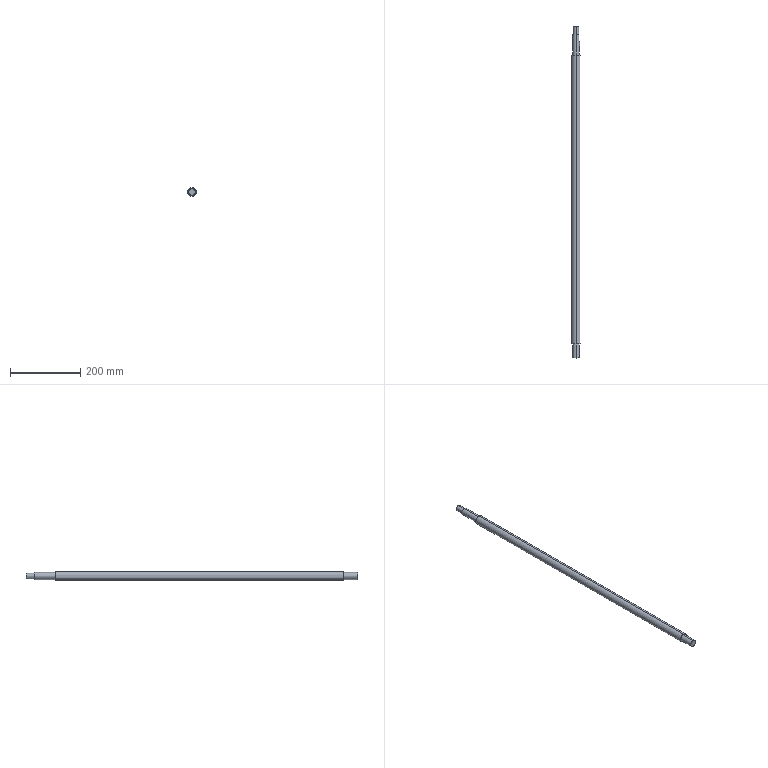Part | STEP file | OT2025004-02-10 Shaft 2 | 1 solid | 28 faces | box 25 x 946 x 25 mm | volume 439586 mm3 | cylinder 12 | cone 9 | plane 7 | commonest cylinder face diameters 2.5 x4 20 x4 16 x2 25 x2
STEP:
#1=CARTESIAN_POINT('',(-0.5,878.75,1.25));
#2=VERTEX_POINT('',#1);
#3=CARTESIAN_POINT('',(-0.5,878.75,-1.25));
#4=VERTEX_POINT('',#3);
#5=CARTESIAN_POINT('',(-0.5,878.75,0.));
#6=DIRECTION('',(1.,0.,0.));
#7=DIRECTION('',(0.,0.,-1.));
#8=AXIS2_PLACEMENT_3D('',#5,#6,#7);
#9=CIRCLE('',#8,1.25);
#10=EDGE_CURVE('',#2,#4,#9,.T.);
#11=ORIENTED_EDGE('',*,*,#10,.F.);
#12=CARTESIAN_POINT('',(8.,878.75,1.25));
#13=VERTEX_POINT('',#12);
#14=CARTESIAN_POINT('',(8.,878.75,1.25));
#15=DIRECTION('',(1.,0.,0.));
#16=VECTOR('',#15,1000.);
#17=LINE('',#14,#16);
#18=EDGE_CURVE('',#2,#13,#17,.T.);
#19=ORIENTED_EDGE('',*,*,#18,.T.);
#20=CARTESIAN_POINT('',(8.,878.75,-1.25));
#21=VERTEX_POINT('',#20);
#22=CARTESIAN_POINT('',(8.,878.75,0.));
#23=DIRECTION('',(1.,0.,0.));
#24=DIRECTION('',(0.,0.,-1.));
#25=AXIS2_PLACEMENT_3D('',#22,#23,#24);
#26=CIRCLE('',#25,1.25);
#27=EDGE_CURVE('',#13,#21,#26,.T.);
#28=ORIENTED_EDGE('',*,*,#27,.T.);
#29=CARTESIAN_POINT('',(8.,878.75,-1.25));
#30=DIRECTION('',(1.,0.,0.));
#31=VECTOR('',#30,1000.);
#32=LINE('',#29,#31);
#33=EDGE_CURVE('',#4,#21,#32,.T.);
#34=ORIENTED_EDGE('',*,*,#33,.F.);
#35=EDGE_LOOP('',(#11,#19,#28,#34));
#36=FACE_OUTER_BOUND('',#35,.T.);
#37=CARTESIAN_POINT('',(8.,878.75,0.));
#38=DIRECTION('',(1.,0.,0.));
#39=DIRECTION('',(0.,0.,-1.));
#40=AXIS2_PLACEMENT_3D('',#37,#38,#39);
#41=CYLINDRICAL_SURFACE('',#40,1.25);
#42=ADVANCED_FACE('',(#36),#41,.F.);
#43=CARTESIAN_POINT('',(-1.222,878.75,0.));
#44=VERTEX_POINT('',#43);
#45=CARTESIAN_POINT('',(-0.5,878.75,-1.25));
#46=DIRECTION('',(0.5,0.,-0.866));
#47=VECTOR('',#46,1000.);
#48=LINE('',#45,#47);
#49=EDGE_CURVE('',#44,#4,#48,.T.);
#50=ORIENTED_EDGE('',*,*,#49,.F.);
#51=CARTESIAN_POINT('',(-0.5,878.75,1.25));
#52=DIRECTION('',(0.5,0.,0.866));
#53=VECTOR('',#52,1000.);
#54=LINE('',#51,#53);
#55=EDGE_CURVE('',#44,#2,#54,.T.);
#56=ORIENTED_EDGE('',*,*,#55,.T.);
#57=ORIENTED_EDGE('',*,*,#10,.T.);
#58=EDGE_LOOP('',(#50,#56,#57));
#59=FACE_OUTER_BOUND('',#58,.T.);
#60=CARTESIAN_POINT('',(-0.5,878.75,0.));
#61=DIRECTION('',(1.,0.,0.));
#62=DIRECTION('',(0.,0.,-1.));
#63=AXIS2_PLACEMENT_3D('',#60,#61,#62);
#64=CONICAL_SURFACE('',#63,1.25,1.047);
#65=ADVANCED_FACE('',(#59),#64,.F.);
#66=CARTESIAN_POINT('',(-0.5,867.25,1.25));
#67=VERTEX_POINT('',#66);
#68=CARTESIAN_POINT('',(-0.5,867.25,-1.25));
#69=VERTEX_POINT('',#68);
#70=CARTESIAN_POINT('',(-0.5,867.25,0.));
#71=DIRECTION('',(1.,0.,0.));
#72=DIRECTION('',(0.,0.,-1.));
#73=AXIS2_PLACEMENT_3D('',#70,#71,#72);
#74=CIRCLE('',#73,1.25);
#75=EDGE_CURVE('',#67,#69,#74,.T.);
#76=ORIENTED_EDGE('',*,*,#75,.F.);
#77=CARTESIAN_POINT('',(8.,867.25,1.25));
#78=VERTEX_POINT('',#77);
#79=CARTESIAN_POINT('',(8.,867.25,1.25));
#80=DIRECTION('',(1.,0.,0.));
#81=VECTOR('',#80,1000.);
#82=LINE('',#79,#81);
#83=EDGE_CURVE('',#67,#78,#82,.T.);
#84=ORIENTED_EDGE('',*,*,#83,.T.);
#85=CARTESIAN_POINT('',(8.,867.25,-1.25));
#86=VERTEX_POINT('',#85);
#87=CARTESIAN_POINT('',(8.,867.25,0.));
#88=DIRECTION('',(1.,0.,0.));
#89=DIRECTION('',(0.,0.,-1.));
#90=AXIS2_PLACEMENT_3D('',#87,#88,#89);
#91=CIRCLE('',#90,1.25);
#92=EDGE_CURVE('',#78,#86,#91,.T.);
#93=ORIENTED_EDGE('',*,*,#92,.T.);
#94=CARTESIAN_POINT('',(8.,867.25,-1.25));
#95=DIRECTION('',(1.,0.,0.));
#96=VECTOR('',#95,1000.);
#97=LINE('',#94,#96);
#98=EDGE_CURVE('',#69,#86,#97,.T.);
#99=ORIENTED_EDGE('',*,*,#98,.F.);
#100=EDGE_LOOP('',(#76,#84,#93,#99));
#101=FACE_OUTER_BOUND('',#100,.T.);
#102=CARTESIAN_POINT('',(8.,867.25,0.));
#103=DIRECTION('',(1.,0.,0.));
#104=DIRECTION('',(0.,0.,-1.));
#105=AXIS2_PLACEMENT_3D('',#102,#103,#104);
#106=CYLINDRICAL_SURFACE('',#105,1.25);
#107=ADVANCED_FACE('',(#101),#106,.F.);
#108=CARTESIAN_POINT('',(-1.222,867.25,0.));
#109=VERTEX_POINT('',#108);
#110=CARTESIAN_POINT('',(-0.5,867.25,-1.25));
#111=DIRECTION('',(0.5,0.,-0.866));
#112=VECTOR('',#111,1000.);
#113=LINE('',#110,#112);
#114=EDGE_CURVE('',#109,#69,#113,.T.);
#115=ORIENTED_EDGE('',*,*,#114,.F.);
#116=CARTESIAN_POINT('',(-0.5,867.25,1.25));
#117=DIRECTION('',(0.5,0.,0.866));
#118=VECTOR('',#117,1000.);
#119=LINE('',#116,#118);
#120=EDGE_CURVE('',#109,#67,#119,.T.);
#121=ORIENTED_EDGE('',*,*,#120,.T.);
#122=ORIENTED_EDGE('',*,*,#75,.T.);
#123=EDGE_LOOP('',(#115,#121,#122));
#124=FACE_OUTER_BOUND('',#123,.T.);
#125=CARTESIAN_POINT('',(-0.5,867.25,0.));
#126=DIRECTION('',(1.,0.,0.));
#127=DIRECTION('',(0.,0.,-1.));
#128=AXIS2_PLACEMENT_3D('',#125,#126,#127);
#129=CONICAL_SURFACE('',#128,1.25,1.047);
#130=ADVANCED_FACE('',(#124),#129,.F.);
#131=CARTESIAN_POINT('',(0.,883.,9.5));
#132=VERTEX_POINT('',#131);
#133=CARTESIAN_POINT('',(8.,883.,5.123));
#134=VERTEX_POINT('',#133);
#135=CARTESIAN_POINT('',(0.,883.,0.));
#136=DIRECTION('',(0.,1.,0.));
#137=DIRECTION('',(0.,0.,1.));
#138=AXIS2_PLACEMENT_3D('',#135,#136,#137);
#139=CIRCLE('',#138,9.5);
#140=EDGE_CURVE('',#132,#134,#139,.T.);
#141=ORIENTED_EDGE('',*,*,#140,.F.);
#142=CARTESIAN_POINT('',(0.,882.5,10.));
#143=VERTEX_POINT('',#142);
#144=CARTESIAN_POINT('',(0.,883.,9.5));
#145=DIRECTION('',(0.,-0.7071,0.7071));
#146=VECTOR('',#145,1000.);
#147=LINE('',#144,#146);
#148=EDGE_CURVE('',#132,#143,#147,.T.);
#149=ORIENTED_EDGE('',*,*,#148,.T.);
#150=CARTESIAN_POINT('',(8.,882.5,6.));
#151=VERTEX_POINT('',#150);
#152=CARTESIAN_POINT('',(0.,882.5,0.));
#153=DIRECTION('',(0.,-1.,0.));
#154=DIRECTION('',(0.,0.,1.));
#155=AXIS2_PLACEMENT_3D('',#152,#153,#154);
#156=CIRCLE('',#155,10.);
#157=EDGE_CURVE('',#151,#143,#156,.T.);
#158=ORIENTED_EDGE('',*,*,#157,.F.);
#159=CARTESIAN_POINT('',(8.,883.,5.123));
#160=CARTESIAN_POINT('',(8.,882.84,5.42));
#161=CARTESIAN_POINT('',(8.,882.673,5.712));
#162=CARTESIAN_POINT('',(8.,882.5,6.));
#163=B_SPLINE_CURVE_WITH_KNOTS('',3,(#159,#160,#161,#162),.UNSPECIFIED.,.F.,.F.,(4,4),(0.02082,0.02183),.UNSPECIFIED.);
#164=EDGE_CURVE('',#134,#151,#163,.T.);
#165=ORIENTED_EDGE('',*,*,#164,.F.);
#166=EDGE_LOOP('',(#141,#149,#158,#165));
#167=FACE_OUTER_BOUND('',#166,.T.);
#168=CARTESIAN_POINT('',(0.,883.,0.));
#169=DIRECTION('',(0.,-1.,0.));
#170=DIRECTION('',(0.,0.,-1.));
#171=AXIS2_PLACEMENT_3D('',#168,#169,#170);
#172=CONICAL_SURFACE('',#171,9.5,0.7854);
#173=ADVANCED_FACE('',(#167),#172,.T.);
#174=ORIENTED_EDGE('',*,*,#148,.F.);
#175=CARTESIAN_POINT('',(0.,883.,-9.5));
#176=VERTEX_POINT('',#175);
#177=CARTESIAN_POINT('',(0.,883.,0.));
#178=DIRECTION('',(0.,1.,0.));
#179=DIRECTION('',(0.,0.,1.));
#180=AXIS2_PLACEMENT_3D('',#177,#178,#179);
#181=CIRCLE('',#180,9.5);
#182=EDGE_CURVE('',#176,#132,#181,.T.);
#183=ORIENTED_EDGE('',*,*,#182,.F.);
#184=CARTESIAN_POINT('',(0.,882.5,-10.));
#185=VERTEX_POINT('',#184);
#186=CARTESIAN_POINT('',(0.,883.,-9.5));
#187=DIRECTION('',(0.,-0.7071,-0.7071));
#188=VECTOR('',#187,1000.);
#189=LINE('',#186,#188);
#190=EDGE_CURVE('',#176,#185,#189,.T.);
#191=ORIENTED_EDGE('',*,*,#190,.T.);
#192=CARTESIAN_POINT('',(0.,882.5,0.));
#193=DIRECTION('',(0.,-1.,0.));
#194=DIRECTION('',(0.,0.,1.));
#195=AXIS2_PLACEMENT_3D('',#192,#193,#194);
#196=CIRCLE('',#195,10.);
#197=EDGE_CURVE('',#143,#185,#196,.T.);
#198=ORIENTED_EDGE('',*,*,#197,.F.);
#199=EDGE_LOOP('',(#174,#183,#191,#198));
#200=FACE_OUTER_BOUND('',#199,.T.);
#201=CARTESIAN_POINT('',(0.,883.,0.));
#202=DIRECTION('',(0.,-1.,0.));
#203=DIRECTION('',(0.,0.,-1.));
#204=AXIS2_PLACEMENT_3D('',#201,#202,#203);
#205=CONICAL_SURFACE('',#204,9.5,0.7854);
#206=ADVANCED_FACE('',(#200),#205,.T.);
#207=CARTESIAN_POINT('',(0.,-40.,-9.5));
#208=VERTEX_POINT('',#207);
#209=CARTESIAN_POINT('',(0.,-40.,9.5));
#210=VERTEX_POINT('',#209);
#211=CARTESIAN_POINT('',(0.,-40.,0.));
#212=DIRECTION('',(0.,-1.,0.));
#213=DIRECTION('',(0.,0.,-1.));
#214=AXIS2_PLACEMENT_3D('',#211,#212,#213);
#215=CIRCLE('',#214,9.5);
#216=EDGE_CURVE('',#208,#210,#215,.T.);
#217=ORIENTED_EDGE('',*,*,#216,.F.);
#218=CARTESIAN_POINT('',(0.,-39.5,-10.));
#219=VERTEX_POINT('',#218);
#220=CARTESIAN_POINT('',(0.,-40.,-9.5));
#221=DIRECTION('',(0.,0.7071,-0.7071));
#222=VECTOR('',#221,1000.);
#223=LINE('',#220,#222);
#224=EDGE_CURVE('',#208,#219,#223,.T.);
#225=ORIENTED_EDGE('',*,*,#224,.T.);
#226=CARTESIAN_POINT('',(0.,-39.5,10.));
#227=VERTEX_POINT('',#226);
#228=CARTESIAN_POINT('',(0.,-39.5,0.));
#229=DIRECTION('',(0.,1.,0.));
#230=DIRECTION('',(0.,0.,-1.));
#231=AXIS2_PLACEMENT_3D('',#228,#229,#230);
#232=CIRCLE('',#231,10.);
#233=EDGE_CURVE('',#227,#219,#232,.T.);
#234=ORIENTED_EDGE('',*,*,#233,.F.);
#235=CARTESIAN_POINT('',(0.,-40.,9.5));
#236=DIRECTION('',(0.,0.7071,0.7071));
#237=VECTOR('',#236,1000.);
#238=LINE('',#235,#237);
#239=EDGE_CURVE('',#210,#227,#238,.T.);
#240=ORIENTED_EDGE('',*,*,#239,.F.);
#241=EDGE_LOOP('',(#217,#225,#234,#240));
#242=FACE_OUTER_BOUND('',#241,.T.);
#243=CARTESIAN_POINT('',(0.,-40.,0.));
#244=DIRECTION('',(0.,1.,0.));
#245=DIRECTION('',(0.,0.,1.));
#246=AXIS2_PLACEMENT_3D('',#243,#244,#245);
#247=CONICAL_SURFACE('',#246,9.5,0.7854);
#248=ADVANCED_FACE('',(#242),#247,.T.);
#249=CARTESIAN_POINT('',(0.,906.,8.));
#250=VERTEX_POINT('',#249);
#251=CARTESIAN_POINT('',(0.,906.,-8.));
#252=VERTEX_POINT('',#251);
#253=CARTESIAN_POINT('',(0.,906.,0.));
#254=DIRECTION('',(0.,1.,0.));
#255=DIRECTION('',(0.,0.,1.));
#256=AXIS2_PLACEMENT_3D('',#253,#254,#255);
#257=CIRCLE('',#256,8.);
#258=EDGE_CURVE('',#250,#252,#257,.T.);
#259=ORIENTED_EDGE('',*,*,#258,.F.);
#260=CARTESIAN_POINT('',(0.,883.,8.));
#261=VERTEX_POINT('',#260);
#262=CARTESIAN_POINT('',(0.,906.,8.));
#263=DIRECTION('',(0.,-1.,0.));
#264=VECTOR('',#263,1000.);
#265=LINE('',#262,#264);
#266=EDGE_CURVE('',#250,#261,#265,.T.);
#267=ORIENTED_EDGE('',*,*,#266,.T.);
#268=CARTESIAN_POINT('',(8.,883.,0.));
#269=VERTEX_POINT('',#268);
#270=CARTESIAN_POINT('',(0.,883.,0.));
#271=DIRECTION('',(0.,1.,0.));
#272=DIRECTION('',(0.,0.,1.));
#273=AXIS2_PLACEMENT_3D('',#270,#271,#272);
#274=CIRCLE('',#273,8.);
#275=EDGE_CURVE('',#261,#269,#274,.T.);
#276=ORIENTED_EDGE('',*,*,#275,.T.);
#277=CARTESIAN_POINT('',(0.,883.,-8.));
#278=VERTEX_POINT('',#277);
#279=CARTESIAN_POINT('',(0.,883.,0.));
#280=DIRECTION('',(0.,1.,0.));
#281=DIRECTION('',(0.,0.,1.));
#282=AXIS2_PLACEMENT_3D('',#279,#280,#281);
#283=CIRCLE('',#282,8.);
#284=EDGE_CURVE('',#269,#278,#283,.T.);
#285=ORIENTED_EDGE('',*,*,#284,.T.);
#286=CARTESIAN_POINT('',(0.,906.,-8.));
#287=DIRECTION('',(0.,-1.,0.));
#288=VECTOR('',#287,1000.);
#289=LINE('',#286,#288);
#290=EDGE_CURVE('',#252,#278,#289,.T.);
#291=ORIENTED_EDGE('',*,*,#290,.F.);
#292=EDGE_LOOP('',(#259,#267,#276,#285,#291));
#293=FACE_OUTER_BOUND('',#292,.T.);
#294=CARTESIAN_POINT('',(0.,906.,0.));
#295=DIRECTION('',(0.,-1.,0.));
#296=DIRECTION('',(0.,0.,-1.));
#297=AXIS2_PLACEMENT_3D('',#294,#295,#296);
#298=CYLINDRICAL_SURFACE('',#297,8.);
#299=ADVANCED_FACE('',(#293),#298,.T.);
#300=ORIENTED_EDGE('',*,*,#233,.T.);
#301=CARTESIAN_POINT('',(0.,0.,-10.));
#302=VERTEX_POINT('',#301);
#303=CARTESIAN_POINT('',(0.,-40.,-10.));
#304=DIRECTION('',(0.,1.,0.));
#305=VECTOR('',#304,1000.);
#306=LINE('',#303,#305);
#307=EDGE_CURVE('',#219,#302,#306,.T.);
#308=ORIENTED_EDGE('',*,*,#307,.T.);
#309=CARTESIAN_POINT('',(0.,0.,10.));
#310=VERTEX_POINT('',#309);
#311=CARTESIAN_POINT('',(0.,0.,0.));
#312=DIRECTION('',(0.,-1.,0.));
#313=DIRECTION('',(0.,0.,-1.));
#314=AXIS2_PLACEMENT_3D('',#311,#312,#313);
#315=CIRCLE('',#314,10.);
#316=EDGE_CURVE('',#302,#310,#315,.T.);
#317=ORIENTED_EDGE('',*,*,#316,.T.);
#318=CARTESIAN_POINT('',(0.,-40.,10.));
#319=DIRECTION('',(0.,1.,0.));
#320=VECTOR('',#319,1000.);
#321=LINE('',#318,#320);
#322=EDGE_CURVE('',#227,#310,#321,.T.);
#323=ORIENTED_EDGE('',*,*,#322,.F.);
#324=EDGE_LOOP('',(#300,#308,#317,#323));
#325=FACE_OUTER_BOUND('',#324,.T.);
#326=CARTESIAN_POINT('',(0.,-40.,0.));
#327=DIRECTION('',(0.,1.,0.));
#328=DIRECTION('',(0.,0.,1.));
#329=AXIS2_PLACEMENT_3D('',#326,#327,#328);
#330=CYLINDRICAL_SURFACE('',#329,10.);
#331=ADVANCED_FACE('',(#325),#330,.T.);
#332=ORIENTED_EDGE('',*,*,#157,.T.);
#333=CARTESIAN_POINT('',(0.,823.,10.));
#334=VERTEX_POINT('',#333);
#335=CARTESIAN_POINT('',(0.,883.,10.));
#336=DIRECTION('',(0.,-1.,0.));
#337=VECTOR('',#336,1000.);
#338=LINE('',#335,#337);
#339=EDGE_CURVE('',#143,#334,#338,.T.);
#340=ORIENTED_EDGE('',*,*,#339,.T.);
#341=CARTESIAN_POINT('',(0.,823.,-10.));
#342=VERTEX_POINT('',#341);
#343=CARTESIAN_POINT('',(0.,823.,0.));
#344=DIRECTION('',(0.,1.,0.));
#345=DIRECTION('',(0.,0.,1.));
#346=AXIS2_PLACEMENT_3D('',#343,#344,#345);
#347=CIRCLE('',#346,10.);
#348=EDGE_CURVE('',#334,#342,#347,.T.);
#349=ORIENTED_EDGE('',*,*,#348,.T.);
#350=CARTESIAN_POINT('',(0.,883.,-10.));
#351=DIRECTION('',(0.,-1.,0.));
#352=VECTOR('',#351,1000.);
#353=LINE('',#350,#352);
#354=EDGE_CURVE('',#185,#342,#353,.T.);
#355=ORIENTED_EDGE('',*,*,#354,.F.);
#356=CARTESIAN_POINT('',(8.,882.5,-6.));
#357=VERTEX_POINT('',#356);
#358=CARTESIAN_POINT('',(0.,882.5,0.));
#359=DIRECTION('',(0.,-1.,0.));
#360=DIRECTION('',(0.,0.,1.));
#361=AXIS2_PLACEMENT_3D('',#358,#359,#360);
#362=CIRCLE('',#361,10.);
#363=EDGE_CURVE('',#185,#357,#362,.T.);
#364=ORIENTED_EDGE('',*,*,#363,.T.);
#365=CARTESIAN_POINT('',(8.,862.,-6.));
#366=VERTEX_POINT('',#365);
#367=CARTESIAN_POINT('',(8.,862.,-6.));
#368=DIRECTION('',(0.,1.,0.));
#369=VECTOR('',#368,1000.);
#370=LINE('',#367,#369);
#371=EDGE_CURVE('',#366,#357,#370,.T.);
#372=ORIENTED_EDGE('',*,*,#371,.F.);
#373=CARTESIAN_POINT('',(8.,862.,6.));
#374=VERTEX_POINT('',#373);
#375=CARTESIAN_POINT('',(0.,862.,0.));
#376=DIRECTION('',(0.,1.,0.));
#377=DIRECTION('',(0.,0.,1.));
#378=AXIS2_PLACEMENT_3D('',#375,#376,#377);
#379=CIRCLE('',#378,10.);
#380=EDGE_CURVE('',#374,#366,#379,.T.);
#381=ORIENTED_EDGE('',*,*,#380,.F.);
#382=CARTESIAN_POINT('',(8.,862.,6.));
#383=DIRECTION('',(0.,1.,0.));
#384=VECTOR('',#383,1000.);
#385=LINE('',#382,#384);
#386=EDGE_CURVE('',#374,#151,#385,.T.);
#387=ORIENTED_EDGE('',*,*,#386,.T.);
#388=EDGE_LOOP('',(#332,#340,#349,#355,#364,#372,#381,#387));
#389=FACE_OUTER_BOUND('',#388,.T.);
#390=CARTESIAN_POINT('',(0.,883.,0.));
#391=DIRECTION('',(0.,-1.,0.));
#392=DIRECTION('',(0.,0.,-1.));
#393=AXIS2_PLACEMENT_3D('',#390,#391,#392);
#394=CYLINDRICAL_SURFACE('',#393,10.);
#395=ADVANCED_FACE('',(#389),#394,.T.);
#396=CARTESIAN_POINT('',(0.,823.,12.5));
#397=VERTEX_POINT('',#396);
#398=CARTESIAN_POINT('',(0.,823.,-12.5));
#399=VERTEX_POINT('',#398);
#400=CARTESIAN_POINT('',(0.,823.,0.));
#401=DIRECTION('',(0.,1.,0.));
#402=DIRECTION('',(0.,0.,1.));
#403=AXIS2_PLACEMENT_3D('',#400,#401,#402);
#404=CIRCLE('',#403,12.5);
#405=EDGE_CURVE('',#397,#399,#404,.T.);
#406=ORIENTED_EDGE('',*,*,#405,.F.);
#407=CARTESIAN_POINT('',(0.,0.,12.5));
#408=VERTEX_POINT('',#407);
#409=CARTESIAN_POINT('',(0.,823.,12.5));
#410=DIRECTION('',(0.,-1.,0.));
#411=VECTOR('',#410,1000.);
#412=LINE('',#409,#411);
#413=EDGE_CURVE('',#397,#408,#412,.T.);
#414=ORIENTED_EDGE('',*,*,#413,.T.);
#415=CARTESIAN_POINT('',(0.,0.,-12.5));
#416=VERTEX_POINT('',#415);
#417=CARTESIAN_POINT('',(0.,0.,0.));
#418=DIRECTION('',(0.,1.,0.));
#419=DIRECTION('',(0.,0.,1.));
#420=AXIS2_PLACEMENT_3D('',#417,#418,#419);
#421=CIRCLE('',#420,12.5);
#422=EDGE_CURVE('',#408,#416,#421,.T.);
#423=ORIENTED_EDGE('',*,*,#422,.T.);
#424=CARTESIAN_POINT('',(0.,823.,-12.5));
#425=DIRECTION('',(0.,-1.,0.));
#426=VECTOR('',#425,1000.);
#427=LINE('',#424,#426);
#428=EDGE_CURVE('',#399,#416,#427,.T.);
#429=ORIENTED_EDGE('',*,*,#428,.F.);
#430=EDGE_LOOP('',(#406,#414,#423,#429));
#431=FACE_OUTER_BOUND('',#430,.T.);
#432=CARTESIAN_POINT('',(0.,823.,0.));
#433=DIRECTION('',(0.,-1.,0.));
#434=DIRECTION('',(0.,0.,-1.));
#435=AXIS2_PLACEMENT_3D('',#432,#433,#434);
#436=CYLINDRICAL_SURFACE('',#435,12.5);
#437=ADVANCED_FACE('',(#431),#436,.T.);
#438=ORIENTED_EDGE('',*,*,#413,.F.);
#439=CARTESIAN_POINT('',(0.,823.,0.));
#440=DIRECTION('',(0.,1.,0.));
#441=DIRECTION('',(0.,0.,1.));
#442=AXIS2_PLACEMENT_3D('',#439,#440,#441);
#443=CIRCLE('',#442,12.5);
#444=EDGE_CURVE('',#399,#397,#443,.T.);
#445=ORIENTED_EDGE('',*,*,#444,.F.);
#446=ORIENTED_EDGE('',*,*,#428,.T.);
#447=CARTESIAN_POINT('',(0.,0.,0.));
#448=DIRECTION('',(0.,1.,0.));
#449=DIRECTION('',(0.,0.,1.));
#450=AXIS2_PLACEMENT_3D('',#447,#448,#449);
#451=CIRCLE('',#450,12.5);
#452=EDGE_CURVE('',#416,#408,#451,.T.);
#453=ORIENTED_EDGE('',*,*,#452,.T.);
#454=EDGE_LOOP('',(#438,#445,#446,#453));
#455=FACE_OUTER_BOUND('',#454,.T.);
#456=CARTESIAN_POINT('',(0.,823.,0.));
#457=DIRECTION('',(0.,-1.,0.));
#458=DIRECTION('',(0.,0.,-1.));
#459=AXIS2_PLACEMENT_3D('',#456,#457,#458);
#460=CYLINDRICAL_SURFACE('',#459,12.5);
#461=ADVANCED_FACE('',(#455),#460,.T.);
#462=CARTESIAN_POINT('',(0.,823.,0.));
#463=DIRECTION('',(0.,1.,0.));
#464=DIRECTION('',(0.,0.,1.));
#465=AXIS2_PLACEMENT_3D('',#462,#463,#464);
#466=CIRCLE('',#465,10.);
#467=EDGE_CURVE('',#342,#334,#466,.T.);
#468=ORIENTED_EDGE('',*,*,#467,.F.);
#469=ORIENTED_EDGE('',*,*,#348,.F.);
#470=EDGE_LOOP('',(#468,#469));
#471=FACE_BOUND('',#470,.T.);
#472=ORIENTED_EDGE('',*,*,#444,.T.);
#473=ORIENTED_EDGE('',*,*,#405,.T.);
#474=EDGE_LOOP('',(#472,#473));
#475=FACE_OUTER_BOUND('',#474,.T.);
#476=CARTESIAN_POINT('',(0.,823.,0.));
#477=DIRECTION('',(0.,1.,0.));
#478=DIRECTION('',(0.,0.,1.));
#479=AXIS2_PLACEMENT_3D('',#476,#477,#478);
#480=PLANE('',#479);
#481=ADVANCED_FACE('',(#471,#475),#480,.T.);
#482=CARTESIAN_POINT('',(0.,0.,0.));
#483=DIRECTION('',(0.,-1.,0.));
#484=DIRECTION('',(0.,0.,-1.));
#485=AXIS2_PLACEMENT_3D('',#482,#483,#484);
#486=CIRCLE('',#485,10.);
#487=EDGE_CURVE('',#310,#302,#486,.T.);
#488=ORIENTED_EDGE('',*,*,#487,.F.);
#489=ORIENTED_EDGE('',*,*,#316,.F.);
#490=EDGE_LOOP('',(#488,#489));
#491=FACE_BOUND('',#490,.T.);
#492=ORIENTED_EDGE('',*,*,#452,.F.);
#493=ORIENTED_EDGE('',*,*,#422,.F.);
#494=EDGE_LOOP('',(#492,#493));
#495=FACE_OUTER_BOUND('',#494,.T.);
#496=CARTESIAN_POINT('',(0.,0.,0.));
#497=DIRECTION('',(0.,1.,0.));
#498=DIRECTION('',(0.,0.,1.));
#499=AXIS2_PLACEMENT_3D('',#496,#497,#498);
#500=PLANE('',#499);
#501=ADVANCED_FACE('',(#491,#495),#500,.F.);
#502=ORIENTED_EDGE('',*,*,#339,.F.);
#503=ORIENTED_EDGE('',*,*,#197,.T.);
#504=ORIENTED_EDGE('',*,*,#354,.T.);
#505=ORIENTED_EDGE('',*,*,#467,.T.);
#506=EDGE_LOOP('',(#502,#503,#504,#505));
#507=FACE_OUTER_BOUND('',#506,.T.);
#508=CARTESIAN_POINT('',(0.,883.,0.));
#509=DIRECTION('',(0.,-1.,0.));
#510=DIRECTION('',(0.,0.,-1.));
#511=AXIS2_PLACEMENT_3D('',#508,#509,#510);
#512=CYLINDRICAL_SURFACE('',#511,10.);
#513=ADVANCED_FACE('',(#507),#512,.T.);
#514=CARTESIAN_POINT('',(8.,883.,-5.123));
#515=VERTEX_POINT('',#514);
#516=CARTESIAN_POINT('',(8.,883.,-6.));
#517=DIRECTION('',(0.,0.,1.));
#518=VECTOR('',#517,1000.);
#519=LINE('',#516,#518);
#520=EDGE_CURVE('',#515,#269,#519,.T.);
#521=ORIENTED_EDGE('',*,*,#520,.F.);
#522=CARTESIAN_POINT('',(0.,883.,0.));
#523=DIRECTION('',(0.,1.,0.));
#524=DIRECTION('',(0.,0.,1.));
#525=AXIS2_PLACEMENT_3D('',#522,#523,#524);
#526=CIRCLE('',#525,9.5);
#527=EDGE_CURVE('',#515,#176,#526,.T.);
#528=ORIENTED_EDGE('',*,*,#527,.T.);
#529=ORIENTED_EDGE('',*,*,#182,.T.);
#530=ORIENTED_EDGE('',*,*,#140,.T.);
#531=CARTESIAN_POINT('',(8.,883.,-6.));
#532=DIRECTION('',(0.,0.,1.));
#533=VECTOR('',#532,1000.);
#534=LINE('',#531,#533);
#535=EDGE_CURVE('',#269,#134,#534,.T.);
#536=ORIENTED_EDGE('',*,*,#535,.F.);
#537=ORIENTED_EDGE('',*,*,#275,.F.);
#538=CARTESIAN_POINT('',(0.,883.,0.));
#539=DIRECTION('',(0.,1.,0.));
#540=DIRECTION('',(0.,0.,1.));
#541=AXIS2_PLACEMENT_3D('',#538,#539,#540);
#542=CIRCLE('',#541,8.);
#543=EDGE_CURVE('',#278,#261,#542,.T.);
#544=ORIENTED_EDGE('',*,*,#543,.F.);
#545=ORIENTED_EDGE('',*,*,#284,.F.);
#546=EDGE_LOOP('',(#521,#528,#529,#530,#536,#537,#544,#545));
#547=FACE_OUTER_BOUND('',#546,.T.);
#548=CARTESIAN_POINT('',(0.,883.,0.));
#549=DIRECTION('',(0.,1.,0.));
#550=DIRECTION('',(0.,0.,1.));
#551=AXIS2_PLACEMENT_3D('',#548,#549,#550);
#552=PLANE('',#551);
#553=ADVANCED_FACE('',(#547),#552,.T.);
#554=ORIENTED_EDGE('',*,*,#307,.F.);
#555=CARTESIAN_POINT('',(0.,-39.5,0.));
#556=DIRECTION('',(0.,1.,0.));
#557=DIRECTION('',(0.,0.,-1.));
#558=AXIS2_PLACEMENT_3D('',#555,#556,#557);
#559=CIRCLE('',#558,10.);
#560=EDGE_CURVE('',#219,#227,#559,.T.);
#561=ORIENTED_EDGE('',*,*,#560,.T.);
#562=ORIENTED_EDGE('',*,*,#322,.T.);
#563=ORIENTED_EDGE('',*,*,#487,.T.);
#564=EDGE_LOOP('',(#554,#561,#562,#563));
#565=FACE_OUTER_BOUND('',#564,.T.);
#566=CARTESIAN_POINT('',(0.,-40.,0.));
#567=DIRECTION('',(0.,1.,0.));
#568=DIRECTION('',(0.,0.,1.));
#569=AXIS2_PLACEMENT_3D('',#566,#567,#568);
#570=CYLINDRICAL_SURFACE('',#569,10.);
#571=ADVANCED_FACE('',(#565),#570,.T.);
#572=CARTESIAN_POINT('',(0.,-40.,0.));
#573=DIRECTION('',(0.,-1.,0.));
#574=DIRECTION('',(0.,0.,-1.));
#575=AXIS2_PLACEMENT_3D('',#572,#573,#574);
#576=CIRCLE('',#575,9.5);
#577=EDGE_CURVE('',#210,#208,#576,.T.);
#578=ORIENTED_EDGE('',*,*,#577,.T.);
#579=ORIENTED_EDGE('',*,*,#216,.T.);
#580=EDGE_LOOP('',(#578,#579));
#581=FACE_OUTER_BOUND('',#580,.T.);
#582=CARTESIAN_POINT('',(0.,-40.,0.));
#583=DIRECTION('',(0.,-1.,0.));
#584=DIRECTION('',(0.,0.,-1.));
#585=AXIS2_PLACEMENT_3D('',#582,#583,#584);
#586=PLANE('',#585);
#587=ADVANCED_FACE('',(#581),#586,.T.);
#588=ORIENTED_EDGE('',*,*,#266,.F.);
#589=CARTESIAN_POINT('',(0.,906.,0.));
#590=DIRECTION('',(0.,1.,0.));
#591=DIRECTION('',(0.,0.,1.));
#592=AXIS2_PLACEMENT_3D('',#589,#590,#591);
#593=CIRCLE('',#592,8.);
#594=EDGE_CURVE('',#252,#250,#593,.T.);
#595=ORIENTED_EDGE('',*,*,#594,.F.);
#596=ORIENTED_EDGE('',*,*,#290,.T.);
#597=ORIENTED_EDGE('',*,*,#543,.T.);
#598=EDGE_LOOP('',(#588,#595,#596,#597));
#599=FACE_OUTER_BOUND('',#598,.T.);
#600=CARTESIAN_POINT('',(0.,906.,0.));
#601=DIRECTION('',(0.,-1.,0.));
#602=DIRECTION('',(0.,0.,-1.));
#603=AXIS2_PLACEMENT_3D('',#600,#601,#602);
#604=CYLINDRICAL_SURFACE('',#603,8.);
#605=ADVANCED_FACE('',(#599),#604,.T.);
#606=ORIENTED_EDGE('',*,*,#594,.T.);
#607=ORIENTED_EDGE('',*,*,#258,.T.);
#608=EDGE_LOOP('',(#606,#607));
#609=FACE_OUTER_BOUND('',#608,.T.);
#610=CARTESIAN_POINT('',(0.,906.,0.));
#611=DIRECTION('',(0.,1.,0.));
#612=DIRECTION('',(0.,0.,1.));
#613=AXIS2_PLACEMENT_3D('',#610,#611,#612);
#614=PLANE('',#613);
#615=ADVANCED_FACE('',(#609),#614,.T.);
#616=ORIENTED_EDGE('',*,*,#224,.F.);
#617=ORIENTED_EDGE('',*,*,#577,.F.);
#618=ORIENTED_EDGE('',*,*,#239,.T.);
#619=ORIENTED_EDGE('',*,*,#560,.F.);
#620=EDGE_LOOP('',(#616,#617,#618,#619));
#621=FACE_OUTER_BOUND('',#620,.T.);
#622=CARTESIAN_POINT('',(0.,-40.,0.));
#623=DIRECTION('',(0.,1.,0.));
#624=DIRECTION('',(0.,0.,1.));
#625=AXIS2_PLACEMENT_3D('',#622,#623,#624);
#626=CONICAL_SURFACE('',#625,9.5,0.7854);
#627=ADVANCED_FACE('',(#621),#626,.T.);
#628=ORIENTED_EDGE('',*,*,#190,.F.);
#629=ORIENTED_EDGE('',*,*,#527,.F.);
#630=CARTESIAN_POINT('',(8.,882.5,-6.));
#631=CARTESIAN_POINT('',(8.,882.673,-5.711));
#632=CARTESIAN_POINT('',(8.,882.84,-5.42));
#633=CARTESIAN_POINT('',(8.,883.,-5.123));
#634=B_SPLINE_CURVE_WITH_KNOTS('',3,(#630,#631,#632,#633),.UNSPECIFIED.,.F.,.F.,(4,4),(0.009044,0.01006),.UNSPECIFIED.);
#635=EDGE_CURVE('',#357,#515,#634,.T.);
#636=ORIENTED_EDGE('',*,*,#635,.F.);
#637=ORIENTED_EDGE('',*,*,#363,.F.);
#638=EDGE_LOOP('',(#628,#629,#636,#637));
#639=FACE_OUTER_BOUND('',#638,.T.);
#640=CARTESIAN_POINT('',(0.,883.,0.));
#641=DIRECTION('',(0.,-1.,0.));
#642=DIRECTION('',(0.,0.,-1.));
#643=AXIS2_PLACEMENT_3D('',#640,#641,#642);
#644=CONICAL_SURFACE('',#643,9.5,0.7854);
#645=ADVANCED_FACE('',(#639),#644,.T.);
#646=CARTESIAN_POINT('',(8.,878.75,0.));
#647=DIRECTION('',(1.,0.,0.));
#648=DIRECTION('',(0.,0.,-1.));
#649=AXIS2_PLACEMENT_3D('',#646,#647,#648);
#650=CIRCLE('',#649,1.25);
#651=EDGE_CURVE('',#21,#13,#650,.T.);
#652=ORIENTED_EDGE('',*,*,#651,.F.);
#653=ORIENTED_EDGE('',*,*,#27,.F.);
#654=EDGE_LOOP('',(#652,#653));
#655=FACE_BOUND('',#654,.T.);
#656=CARTESIAN_POINT('',(8.,867.25,0.));
#657=DIRECTION('',(1.,0.,0.));
#658=DIRECTION('',(0.,0.,-1.));
#659=AXIS2_PLACEMENT_3D('',#656,#657,#658);
#660=CIRCLE('',#659,1.25);
#661=EDGE_CURVE('',#86,#78,#660,.T.);
#662=ORIENTED_EDGE('',*,*,#661,.F.);
#663=ORIENTED_EDGE('',*,*,#92,.F.);
#664=EDGE_LOOP('',(#662,#663));
#665=FACE_BOUND('',#664,.T.);
#666=ORIENTED_EDGE('',*,*,#635,.T.);
#667=ORIENTED_EDGE('',*,*,#520,.T.);
#668=ORIENTED_EDGE('',*,*,#535,.T.);
#669=ORIENTED_EDGE('',*,*,#164,.T.);
#670=ORIENTED_EDGE('',*,*,#386,.F.);
#671=CARTESIAN_POINT('',(8.,862.,-6.));
#672=DIRECTION('',(0.,0.,1.));
#673=VECTOR('',#672,1000.);
#674=LINE('',#671,#673);
#675=EDGE_CURVE('',#366,#374,#674,.T.);
#676=ORIENTED_EDGE('',*,*,#675,.F.);
#677=ORIENTED_EDGE('',*,*,#371,.T.);
#678=EDGE_LOOP('',(#666,#667,#668,#669,#670,#676,#677));
#679=FACE_OUTER_BOUND('',#678,.T.);
#680=CARTESIAN_POINT('',(8.,862.,-6.));
#681=DIRECTION('',(-1.,0.,0.));
#682=DIRECTION('',(0.,0.,1.));
#683=AXIS2_PLACEMENT_3D('',#680,#681,#682);
#684=PLANE('',#683);
#685=ADVANCED_FACE('',(#655,#665,#679),#684,.F.);
#686=ORIENTED_EDGE('',*,*,#380,.T.);
#687=ORIENTED_EDGE('',*,*,#675,.T.);
#688=EDGE_LOOP('',(#686,#687));
#689=FACE_OUTER_BOUND('',#688,.T.);
#690=CARTESIAN_POINT('',(0.,862.,0.));
#691=DIRECTION('',(0.,1.,0.));
#692=DIRECTION('',(0.,0.,1.));
#693=AXIS2_PLACEMENT_3D('',#690,#691,#692);
#694=PLANE('',#693);
#695=ADVANCED_FACE('',(#689),#694,.T.);
#696=ORIENTED_EDGE('',*,*,#120,.F.);
#697=ORIENTED_EDGE('',*,*,#114,.T.);
#698=CARTESIAN_POINT('',(-0.5,867.25,0.));
#699=DIRECTION('',(1.,0.,0.));
#700=DIRECTION('',(0.,0.,-1.));
#701=AXIS2_PLACEMENT_3D('',#698,#699,#700);
#702=CIRCLE('',#701,1.25);
#703=EDGE_CURVE('',#69,#67,#702,.T.);
#704=ORIENTED_EDGE('',*,*,#703,.T.);
#705=EDGE_LOOP('',(#696,#697,#704));
#706=FACE_OUTER_BOUND('',#705,.T.);
#707=CARTESIAN_POINT('',(-0.5,867.25,0.));
#708=DIRECTION('',(1.,0.,0.));
#709=DIRECTION('',(0.,0.,-1.));
#710=AXIS2_PLACEMENT_3D('',#707,#708,#709);
#711=CONICAL_SURFACE('',#710,1.25,1.047);
#712=ADVANCED_FACE('',(#706),#711,.F.);
#713=ORIENTED_EDGE('',*,*,#83,.F.);
#714=ORIENTED_EDGE('',*,*,#703,.F.);
#715=ORIENTED_EDGE('',*,*,#98,.T.);
#716=ORIENTED_EDGE('',*,*,#661,.T.);
#717=EDGE_LOOP('',(#713,#714,#715,#716));
#718=FACE_OUTER_BOUND('',#717,.T.);
#719=CARTESIAN_POINT('',(8.,867.25,0.));
#720=DIRECTION('',(1.,0.,0.));
#721=DIRECTION('',(0.,0.,-1.));
#722=AXIS2_PLACEMENT_3D('',#719,#720,#721);
#723=CYLINDRICAL_SURFACE('',#722,1.25);
#724=ADVANCED_FACE('',(#718),#723,.F.);
#725=ORIENTED_EDGE('',*,*,#55,.F.);
#726=ORIENTED_EDGE('',*,*,#49,.T.);
#727=CARTESIAN_POINT('',(-0.5,878.75,0.));
#728=DIRECTION('',(1.,0.,0.));
#729=DIRECTION('',(0.,0.,-1.));
#730=AXIS2_PLACEMENT_3D('',#727,#728,#729);
#731=CIRCLE('',#730,1.25);
#732=EDGE_CURVE('',#4,#2,#731,.T.);
#733=ORIENTED_EDGE('',*,*,#732,.T.);
#734=EDGE_LOOP('',(#725,#726,#733));
#735=FACE_OUTER_BOUND('',#734,.T.);
#736=CARTESIAN_POINT('',(-0.5,878.75,0.));
#737=DIRECTION('',(1.,0.,0.));
#738=DIRECTION('',(0.,0.,-1.));
#739=AXIS2_PLACEMENT_3D('',#736,#737,#738);
#740=CONICAL_SURFACE('',#739,1.25,1.047);
#741=ADVANCED_FACE('',(#735),#740,.F.);
#742=ORIENTED_EDGE('',*,*,#18,.F.);
#743=ORIENTED_EDGE('',*,*,#732,.F.);
#744=ORIENTED_EDGE('',*,*,#33,.T.);
#745=ORIENTED_EDGE('',*,*,#651,.T.);
#746=EDGE_LOOP('',(#742,#743,#744,#745));
#747=FACE_OUTER_BOUND('',#746,.T.);
#748=CARTESIAN_POINT('',(8.,878.75,0.));
#749=DIRECTION('',(1.,0.,0.));
#750=DIRECTION('',(0.,0.,-1.));
#751=AXIS2_PLACEMENT_3D('',#748,#749,#750);
#752=CYLINDRICAL_SURFACE('',#751,1.25);
#753=ADVANCED_FACE('',(#747),#752,.F.);
#754=CLOSED_SHELL('',(#42,#65,#107,#130,#173,#206,#248,#299,#331,#395,#437,#461,#481,#501,#513,#553,#571,#587,#605,#615,#627,#645,#685,#695,#712,#724,#741,#753));
#755=MANIFOLD_SOLID_BREP('',#754);
#756=CARTESIAN_POINT('',(0.,0.,0.));
#757=DIRECTION('',(0.,0.,1.));
#758=DIRECTION('',(1.,0.,0.));
#759=AXIS2_PLACEMENT_3D('',#756,#757,#758);
#760=(LENGTH_UNIT()NAMED_UNIT(*)SI_UNIT(.MILLI.,.METRE.));
#761=UNCERTAINTY_MEASURE_WITH_UNIT(LENGTH_MEASURE(0.00001),#760,'','');
#762=(NAMED_UNIT(*)PLANE_ANGLE_UNIT()SI_UNIT($,.RADIAN.));
#763=(NAMED_UNIT(*)SI_UNIT($,.STERADIAN.)SOLID_ANGLE_UNIT());
#764=(GEOMETRIC_REPRESENTATION_CONTEXT(3)GLOBAL_UNCERTAINTY_ASSIGNED_CONTEXT((#761))GLOBAL_UNIT_ASSIGNED_CONTEXT((#760,#762,#763))REPRESENTATION_CONTEXT('',''));
#765=ADVANCED_BREP_SHAPE_REPRESENTATION('',(#755,#759),#764);